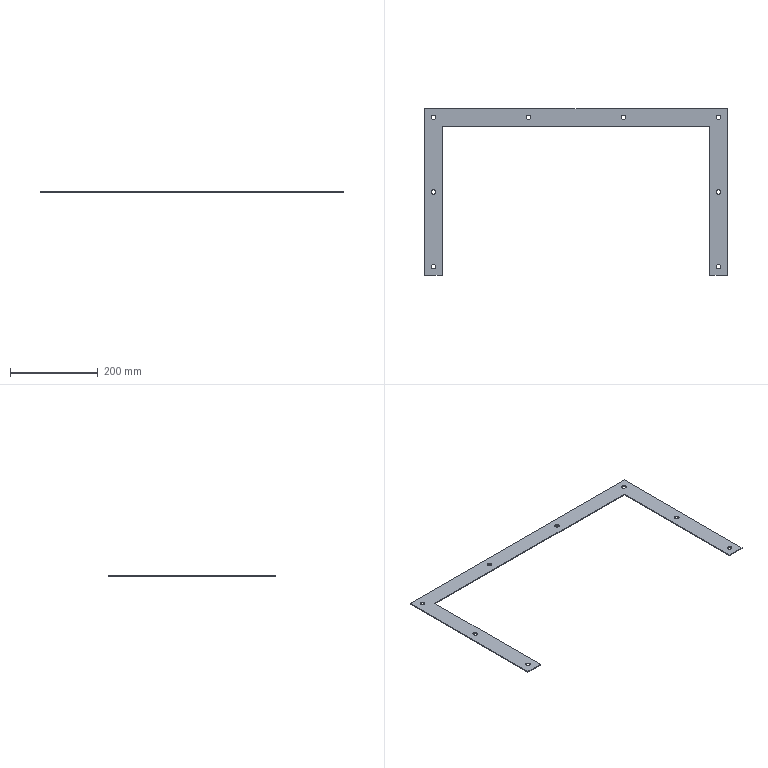Part | STEP file | 750038473 | 1 solid | 26 faces | box 690 x 380 x 2 mm | volume 108343 mm3 | cylinder 16 | plane 10 | commonest cylinder face diameters 10 x16
STEP:
#1=CARTESIAN_POINT('',(330.,275.,2.));
#2=VERTEX_POINT('',#1);
#3=CARTESIAN_POINT('',(320.,275.,2.));
#4=VERTEX_POINT('',#3);
#5=CARTESIAN_POINT('',(325.,275.,2.));
#6=DIRECTION('',(0.,0.,-1.));
#7=DIRECTION('',(-1.,0.,0.));
#8=AXIS2_PLACEMENT_3D('',#5,#6,#7);
#9=CIRCLE('',#8,5.);
#10=EDGE_CURVE('',#2,#4,#9,.T.);
#11=ORIENTED_EDGE('',*,*,#10,.F.);
#12=CARTESIAN_POINT('',(330.,275.,0.));
#13=VERTEX_POINT('',#12);
#14=CARTESIAN_POINT('',(330.,275.,787.721));
#15=DIRECTION('',(0.,0.,-1.));
#16=VECTOR('',#15,1000.);
#17=LINE('',#14,#16);
#18=EDGE_CURVE('',#2,#13,#17,.T.);
#19=ORIENTED_EDGE('',*,*,#18,.T.);
#20=CARTESIAN_POINT('',(320.,275.,0.));
#21=VERTEX_POINT('',#20);
#22=CARTESIAN_POINT('',(325.,275.,0.));
#23=DIRECTION('',(0.,0.,1.));
#24=DIRECTION('',(-1.,0.,0.));
#25=AXIS2_PLACEMENT_3D('',#22,#23,#24);
#26=CIRCLE('',#25,5.);
#27=EDGE_CURVE('',#21,#13,#26,.T.);
#28=ORIENTED_EDGE('',*,*,#27,.F.);
#29=CARTESIAN_POINT('',(320.,275.,787.721));
#30=DIRECTION('',(0.,0.,-1.));
#31=VECTOR('',#30,1000.);
#32=LINE('',#29,#31);
#33=EDGE_CURVE('',#4,#21,#32,.T.);
#34=ORIENTED_EDGE('',*,*,#33,.F.);
#35=EDGE_LOOP('',(#11,#19,#28,#34));
#36=FACE_OUTER_BOUND('',#35,.T.);
#37=CARTESIAN_POINT('',(325.,275.,787.721));
#38=DIRECTION('',(0.,0.,-1.));
#39=DIRECTION('',(-1.,0.,0.));
#40=AXIS2_PLACEMENT_3D('',#37,#38,#39);
#41=CYLINDRICAL_SURFACE('',#40,5.);
#42=ADVANCED_FACE('',(#36),#41,.F.);
#43=CARTESIAN_POINT('',(330.,105.,2.));
#44=VERTEX_POINT('',#43);
#45=CARTESIAN_POINT('',(320.,105.,2.));
#46=VERTEX_POINT('',#45);
#47=CARTESIAN_POINT('',(325.,105.,2.));
#48=DIRECTION('',(0.,0.,-1.));
#49=DIRECTION('',(-1.,0.,0.));
#50=AXIS2_PLACEMENT_3D('',#47,#48,#49);
#51=CIRCLE('',#50,5.);
#52=EDGE_CURVE('',#44,#46,#51,.T.);
#53=ORIENTED_EDGE('',*,*,#52,.F.);
#54=CARTESIAN_POINT('',(330.,105.,0.));
#55=VERTEX_POINT('',#54);
#56=CARTESIAN_POINT('',(330.,105.,787.721));
#57=DIRECTION('',(0.,0.,-1.));
#58=VECTOR('',#57,1000.);
#59=LINE('',#56,#58);
#60=EDGE_CURVE('',#44,#55,#59,.T.);
#61=ORIENTED_EDGE('',*,*,#60,.T.);
#62=CARTESIAN_POINT('',(320.,105.,0.));
#63=VERTEX_POINT('',#62);
#64=CARTESIAN_POINT('',(325.,105.,0.));
#65=DIRECTION('',(0.,0.,1.));
#66=DIRECTION('',(-1.,0.,0.));
#67=AXIS2_PLACEMENT_3D('',#64,#65,#66);
#68=CIRCLE('',#67,5.);
#69=EDGE_CURVE('',#63,#55,#68,.T.);
#70=ORIENTED_EDGE('',*,*,#69,.F.);
#71=CARTESIAN_POINT('',(320.,105.,787.721));
#72=DIRECTION('',(0.,0.,-1.));
#73=VECTOR('',#72,1000.);
#74=LINE('',#71,#73);
#75=EDGE_CURVE('',#46,#63,#74,.T.);
#76=ORIENTED_EDGE('',*,*,#75,.F.);
#77=EDGE_LOOP('',(#53,#61,#70,#76));
#78=FACE_OUTER_BOUND('',#77,.T.);
#79=CARTESIAN_POINT('',(325.,105.,787.721));
#80=DIRECTION('',(0.,0.,-1.));
#81=DIRECTION('',(-1.,0.,0.));
#82=AXIS2_PLACEMENT_3D('',#79,#80,#81);
#83=CYLINDRICAL_SURFACE('',#82,5.);
#84=ADVANCED_FACE('',(#78),#83,.F.);
#85=CARTESIAN_POINT('',(330.,-65.,2.));
#86=VERTEX_POINT('',#85);
#87=CARTESIAN_POINT('',(320.,-65.,2.));
#88=VERTEX_POINT('',#87);
#89=CARTESIAN_POINT('',(325.,-65.,2.));
#90=DIRECTION('',(0.,0.,-1.));
#91=DIRECTION('',(-1.,0.,0.));
#92=AXIS2_PLACEMENT_3D('',#89,#90,#91);
#93=CIRCLE('',#92,5.);
#94=EDGE_CURVE('',#86,#88,#93,.T.);
#95=ORIENTED_EDGE('',*,*,#94,.F.);
#96=CARTESIAN_POINT('',(330.,-65.,0.));
#97=VERTEX_POINT('',#96);
#98=CARTESIAN_POINT('',(330.,-65.,787.721));
#99=DIRECTION('',(0.,0.,-1.));
#100=VECTOR('',#99,1000.);
#101=LINE('',#98,#100);
#102=EDGE_CURVE('',#86,#97,#101,.T.);
#103=ORIENTED_EDGE('',*,*,#102,.T.);
#104=CARTESIAN_POINT('',(320.,-65.,0.));
#105=VERTEX_POINT('',#104);
#106=CARTESIAN_POINT('',(325.,-65.,0.));
#107=DIRECTION('',(0.,0.,1.));
#108=DIRECTION('',(-1.,0.,0.));
#109=AXIS2_PLACEMENT_3D('',#106,#107,#108);
#110=CIRCLE('',#109,5.);
#111=EDGE_CURVE('',#105,#97,#110,.T.);
#112=ORIENTED_EDGE('',*,*,#111,.F.);
#113=CARTESIAN_POINT('',(320.,-65.,787.721));
#114=DIRECTION('',(0.,0.,-1.));
#115=VECTOR('',#114,1000.);
#116=LINE('',#113,#115);
#117=EDGE_CURVE('',#88,#105,#116,.T.);
#118=ORIENTED_EDGE('',*,*,#117,.F.);
#119=EDGE_LOOP('',(#95,#103,#112,#118));
#120=FACE_OUTER_BOUND('',#119,.T.);
#121=CARTESIAN_POINT('',(325.,-65.,787.721));
#122=DIRECTION('',(0.,0.,-1.));
#123=DIRECTION('',(-1.,0.,0.));
#124=AXIS2_PLACEMENT_3D('',#121,#122,#123);
#125=CYLINDRICAL_SURFACE('',#124,5.);
#126=ADVANCED_FACE('',(#120),#125,.F.);
#127=CARTESIAN_POINT('',(113.333,275.,2.));
#128=VERTEX_POINT('',#127);
#129=CARTESIAN_POINT('',(103.333,275.,2.));
#130=VERTEX_POINT('',#129);
#131=CARTESIAN_POINT('',(108.333,275.,2.));
#132=DIRECTION('',(0.,0.,-1.));
#133=DIRECTION('',(-1.,0.,0.));
#134=AXIS2_PLACEMENT_3D('',#131,#132,#133);
#135=CIRCLE('',#134,5.);
#136=EDGE_CURVE('',#128,#130,#135,.T.);
#137=ORIENTED_EDGE('',*,*,#136,.F.);
#138=CARTESIAN_POINT('',(113.333,275.,0.));
#139=VERTEX_POINT('',#138);
#140=CARTESIAN_POINT('',(113.333,275.,787.721));
#141=DIRECTION('',(0.,0.,-1.));
#142=VECTOR('',#141,1000.);
#143=LINE('',#140,#142);
#144=EDGE_CURVE('',#128,#139,#143,.T.);
#145=ORIENTED_EDGE('',*,*,#144,.T.);
#146=CARTESIAN_POINT('',(103.333,275.,0.));
#147=VERTEX_POINT('',#146);
#148=CARTESIAN_POINT('',(108.333,275.,0.));
#149=DIRECTION('',(0.,0.,1.));
#150=DIRECTION('',(-1.,0.,0.));
#151=AXIS2_PLACEMENT_3D('',#148,#149,#150);
#152=CIRCLE('',#151,5.);
#153=EDGE_CURVE('',#147,#139,#152,.T.);
#154=ORIENTED_EDGE('',*,*,#153,.F.);
#155=CARTESIAN_POINT('',(103.333,275.,787.721));
#156=DIRECTION('',(0.,0.,-1.));
#157=VECTOR('',#156,1000.);
#158=LINE('',#155,#157);
#159=EDGE_CURVE('',#130,#147,#158,.T.);
#160=ORIENTED_EDGE('',*,*,#159,.F.);
#161=EDGE_LOOP('',(#137,#145,#154,#160));
#162=FACE_OUTER_BOUND('',#161,.T.);
#163=CARTESIAN_POINT('',(108.333,275.,787.721));
#164=DIRECTION('',(0.,0.,-1.));
#165=DIRECTION('',(-1.,0.,0.));
#166=AXIS2_PLACEMENT_3D('',#163,#164,#165);
#167=CYLINDRICAL_SURFACE('',#166,5.);
#168=ADVANCED_FACE('',(#162),#167,.F.);
#169=CARTESIAN_POINT('',(-103.333,275.,2.));
#170=VERTEX_POINT('',#169);
#171=CARTESIAN_POINT('',(-113.333,275.,2.));
#172=VERTEX_POINT('',#171);
#173=CARTESIAN_POINT('',(-108.333,275.,2.));
#174=DIRECTION('',(0.,0.,-1.));
#175=DIRECTION('',(-1.,0.,0.));
#176=AXIS2_PLACEMENT_3D('',#173,#174,#175);
#177=CIRCLE('',#176,5.);
#178=EDGE_CURVE('',#170,#172,#177,.T.);
#179=ORIENTED_EDGE('',*,*,#178,.F.);
#180=CARTESIAN_POINT('',(-103.333,275.,0.));
#181=VERTEX_POINT('',#180);
#182=CARTESIAN_POINT('',(-103.333,275.,787.721));
#183=DIRECTION('',(0.,0.,-1.));
#184=VECTOR('',#183,1000.);
#185=LINE('',#182,#184);
#186=EDGE_CURVE('',#170,#181,#185,.T.);
#187=ORIENTED_EDGE('',*,*,#186,.T.);
#188=CARTESIAN_POINT('',(-113.333,275.,0.));
#189=VERTEX_POINT('',#188);
#190=CARTESIAN_POINT('',(-108.333,275.,0.));
#191=DIRECTION('',(0.,0.,1.));
#192=DIRECTION('',(-1.,0.,0.));
#193=AXIS2_PLACEMENT_3D('',#190,#191,#192);
#194=CIRCLE('',#193,5.);
#195=EDGE_CURVE('',#189,#181,#194,.T.);
#196=ORIENTED_EDGE('',*,*,#195,.F.);
#197=CARTESIAN_POINT('',(-113.333,275.,787.721));
#198=DIRECTION('',(0.,0.,-1.));
#199=VECTOR('',#198,1000.);
#200=LINE('',#197,#199);
#201=EDGE_CURVE('',#172,#189,#200,.T.);
#202=ORIENTED_EDGE('',*,*,#201,.F.);
#203=EDGE_LOOP('',(#179,#187,#196,#202));
#204=FACE_OUTER_BOUND('',#203,.T.);
#205=CARTESIAN_POINT('',(-108.333,275.,787.721));
#206=DIRECTION('',(0.,0.,-1.));
#207=DIRECTION('',(-1.,0.,0.));
#208=AXIS2_PLACEMENT_3D('',#205,#206,#207);
#209=CYLINDRICAL_SURFACE('',#208,5.);
#210=ADVANCED_FACE('',(#204),#209,.F.);
#211=CARTESIAN_POINT('',(-320.,275.,2.));
#212=VERTEX_POINT('',#211);
#213=CARTESIAN_POINT('',(-330.,275.,2.));
#214=VERTEX_POINT('',#213);
#215=CARTESIAN_POINT('',(-325.,275.,2.));
#216=DIRECTION('',(0.,0.,-1.));
#217=DIRECTION('',(-1.,0.,0.));
#218=AXIS2_PLACEMENT_3D('',#215,#216,#217);
#219=CIRCLE('',#218,5.);
#220=EDGE_CURVE('',#212,#214,#219,.T.);
#221=ORIENTED_EDGE('',*,*,#220,.F.);
#222=CARTESIAN_POINT('',(-320.,275.,0.));
#223=VERTEX_POINT('',#222);
#224=CARTESIAN_POINT('',(-320.,275.,787.721));
#225=DIRECTION('',(0.,0.,-1.));
#226=VECTOR('',#225,1000.);
#227=LINE('',#224,#226);
#228=EDGE_CURVE('',#212,#223,#227,.T.);
#229=ORIENTED_EDGE('',*,*,#228,.T.);
#230=CARTESIAN_POINT('',(-330.,275.,0.));
#231=VERTEX_POINT('',#230);
#232=CARTESIAN_POINT('',(-325.,275.,0.));
#233=DIRECTION('',(0.,0.,1.));
#234=DIRECTION('',(-1.,0.,0.));
#235=AXIS2_PLACEMENT_3D('',#232,#233,#234);
#236=CIRCLE('',#235,5.);
#237=EDGE_CURVE('',#231,#223,#236,.T.);
#238=ORIENTED_EDGE('',*,*,#237,.F.);
#239=CARTESIAN_POINT('',(-330.,275.,787.721));
#240=DIRECTION('',(0.,0.,-1.));
#241=VECTOR('',#240,1000.);
#242=LINE('',#239,#241);
#243=EDGE_CURVE('',#214,#231,#242,.T.);
#244=ORIENTED_EDGE('',*,*,#243,.F.);
#245=EDGE_LOOP('',(#221,#229,#238,#244));
#246=FACE_OUTER_BOUND('',#245,.T.);
#247=CARTESIAN_POINT('',(-325.,275.,787.721));
#248=DIRECTION('',(0.,0.,-1.));
#249=DIRECTION('',(-1.,0.,0.));
#250=AXIS2_PLACEMENT_3D('',#247,#248,#249);
#251=CYLINDRICAL_SURFACE('',#250,5.);
#252=ADVANCED_FACE('',(#246),#251,.F.);
#253=CARTESIAN_POINT('',(-320.,105.,2.));
#254=VERTEX_POINT('',#253);
#255=CARTESIAN_POINT('',(-330.,105.,2.));
#256=VERTEX_POINT('',#255);
#257=CARTESIAN_POINT('',(-325.,105.,2.));
#258=DIRECTION('',(0.,0.,-1.));
#259=DIRECTION('',(-1.,0.,0.));
#260=AXIS2_PLACEMENT_3D('',#257,#258,#259);
#261=CIRCLE('',#260,5.);
#262=EDGE_CURVE('',#254,#256,#261,.T.);
#263=ORIENTED_EDGE('',*,*,#262,.F.);
#264=CARTESIAN_POINT('',(-320.,105.,0.));
#265=VERTEX_POINT('',#264);
#266=CARTESIAN_POINT('',(-320.,105.,787.721));
#267=DIRECTION('',(0.,0.,-1.));
#268=VECTOR('',#267,1000.);
#269=LINE('',#266,#268);
#270=EDGE_CURVE('',#254,#265,#269,.T.);
#271=ORIENTED_EDGE('',*,*,#270,.T.);
#272=CARTESIAN_POINT('',(-330.,105.,0.));
#273=VERTEX_POINT('',#272);
#274=CARTESIAN_POINT('',(-325.,105.,0.));
#275=DIRECTION('',(0.,0.,1.));
#276=DIRECTION('',(-1.,0.,0.));
#277=AXIS2_PLACEMENT_3D('',#274,#275,#276);
#278=CIRCLE('',#277,5.);
#279=EDGE_CURVE('',#273,#265,#278,.T.);
#280=ORIENTED_EDGE('',*,*,#279,.F.);
#281=CARTESIAN_POINT('',(-330.,105.,787.721));
#282=DIRECTION('',(0.,0.,-1.));
#283=VECTOR('',#282,1000.);
#284=LINE('',#281,#283);
#285=EDGE_CURVE('',#256,#273,#284,.T.);
#286=ORIENTED_EDGE('',*,*,#285,.F.);
#287=EDGE_LOOP('',(#263,#271,#280,#286));
#288=FACE_OUTER_BOUND('',#287,.T.);
#289=CARTESIAN_POINT('',(-325.,105.,787.721));
#290=DIRECTION('',(0.,0.,-1.));
#291=DIRECTION('',(-1.,0.,0.));
#292=AXIS2_PLACEMENT_3D('',#289,#290,#291);
#293=CYLINDRICAL_SURFACE('',#292,5.);
#294=ADVANCED_FACE('',(#288),#293,.F.);
#295=CARTESIAN_POINT('',(-320.,-65.,2.));
#296=VERTEX_POINT('',#295);
#297=CARTESIAN_POINT('',(-330.,-65.,2.));
#298=VERTEX_POINT('',#297);
#299=CARTESIAN_POINT('',(-325.,-65.,2.));
#300=DIRECTION('',(0.,0.,-1.));
#301=DIRECTION('',(-1.,0.,0.));
#302=AXIS2_PLACEMENT_3D('',#299,#300,#301);
#303=CIRCLE('',#302,5.);
#304=EDGE_CURVE('',#296,#298,#303,.T.);
#305=ORIENTED_EDGE('',*,*,#304,.F.);
#306=CARTESIAN_POINT('',(-320.,-65.,0.));
#307=VERTEX_POINT('',#306);
#308=CARTESIAN_POINT('',(-320.,-65.,787.721));
#309=DIRECTION('',(0.,0.,-1.));
#310=VECTOR('',#309,1000.);
#311=LINE('',#308,#310);
#312=EDGE_CURVE('',#296,#307,#311,.T.);
#313=ORIENTED_EDGE('',*,*,#312,.T.);
#314=CARTESIAN_POINT('',(-330.,-65.,0.));
#315=VERTEX_POINT('',#314);
#316=CARTESIAN_POINT('',(-325.,-65.,0.));
#317=DIRECTION('',(0.,0.,1.));
#318=DIRECTION('',(-1.,0.,0.));
#319=AXIS2_PLACEMENT_3D('',#316,#317,#318);
#320=CIRCLE('',#319,5.);
#321=EDGE_CURVE('',#315,#307,#320,.T.);
#322=ORIENTED_EDGE('',*,*,#321,.F.);
#323=CARTESIAN_POINT('',(-330.,-65.,787.721));
#324=DIRECTION('',(0.,0.,-1.));
#325=VECTOR('',#324,1000.);
#326=LINE('',#323,#325);
#327=EDGE_CURVE('',#298,#315,#326,.T.);
#328=ORIENTED_EDGE('',*,*,#327,.F.);
#329=EDGE_LOOP('',(#305,#313,#322,#328));
#330=FACE_OUTER_BOUND('',#329,.T.);
#331=CARTESIAN_POINT('',(-325.,-65.,787.721));
#332=DIRECTION('',(0.,0.,-1.));
#333=DIRECTION('',(-1.,0.,0.));
#334=AXIS2_PLACEMENT_3D('',#331,#332,#333);
#335=CYLINDRICAL_SURFACE('',#334,5.);
#336=ADVANCED_FACE('',(#330),#335,.F.);
#337=CARTESIAN_POINT('',(305.,-85.,2.));
#338=VERTEX_POINT('',#337);
#339=CARTESIAN_POINT('',(345.,-85.,2.));
#340=VERTEX_POINT('',#339);
#341=CARTESIAN_POINT('',(0.,-85.,2.));
#342=DIRECTION('',(1.,0.,0.));
#343=VECTOR('',#342,1000.);
#344=LINE('',#341,#343);
#345=EDGE_CURVE('',#338,#340,#344,.T.);
#346=ORIENTED_EDGE('',*,*,#345,.T.);
#347=CARTESIAN_POINT('',(345.,295.,2.));
#348=VERTEX_POINT('',#347);
#349=CARTESIAN_POINT('',(345.,0.,2.));
#350=DIRECTION('',(0.,1.,0.));
#351=VECTOR('',#350,1000.);
#352=LINE('',#349,#351);
#353=EDGE_CURVE('',#340,#348,#352,.T.);
#354=ORIENTED_EDGE('',*,*,#353,.T.);
#355=CARTESIAN_POINT('',(-345.,295.,2.));
#356=VERTEX_POINT('',#355);
#357=CARTESIAN_POINT('',(0.,295.,2.));
#358=DIRECTION('',(-1.,0.,0.));
#359=VECTOR('',#358,1000.);
#360=LINE('',#357,#359);
#361=EDGE_CURVE('',#348,#356,#360,.T.);
#362=ORIENTED_EDGE('',*,*,#361,.T.);
#363=CARTESIAN_POINT('',(-345.,-85.,2.));
#364=VERTEX_POINT('',#363);
#365=CARTESIAN_POINT('',(-345.,0.,2.));
#366=DIRECTION('',(0.,-1.,0.));
#367=VECTOR('',#366,1000.);
#368=LINE('',#365,#367);
#369=EDGE_CURVE('',#356,#364,#368,.T.);
#370=ORIENTED_EDGE('',*,*,#369,.T.);
#371=CARTESIAN_POINT('',(-305.,-85.,2.));
#372=VERTEX_POINT('',#371);
#373=CARTESIAN_POINT('',(0.,-85.,2.));
#374=DIRECTION('',(1.,0.,0.));
#375=VECTOR('',#374,1000.);
#376=LINE('',#373,#375);
#377=EDGE_CURVE('',#364,#372,#376,.T.);
#378=ORIENTED_EDGE('',*,*,#377,.T.);
#379=CARTESIAN_POINT('',(-305.,255.,2.));
#380=VERTEX_POINT('',#379);
#381=CARTESIAN_POINT('',(-305.,0.,2.));
#382=DIRECTION('',(0.,1.,0.));
#383=VECTOR('',#382,1000.);
#384=LINE('',#381,#383);
#385=EDGE_CURVE('',#372,#380,#384,.T.);
#386=ORIENTED_EDGE('',*,*,#385,.T.);
#387=CARTESIAN_POINT('',(305.,255.,2.));
#388=VERTEX_POINT('',#387);
#389=CARTESIAN_POINT('',(0.,255.,2.));
#390=DIRECTION('',(1.,0.,0.));
#391=VECTOR('',#390,1000.);
#392=LINE('',#389,#391);
#393=EDGE_CURVE('',#380,#388,#392,.T.);
#394=ORIENTED_EDGE('',*,*,#393,.T.);
#395=CARTESIAN_POINT('',(305.,0.,2.));
#396=DIRECTION('',(0.,-1.,0.));
#397=VECTOR('',#396,1000.);
#398=LINE('',#395,#397);
#399=EDGE_CURVE('',#388,#338,#398,.T.);
#400=ORIENTED_EDGE('',*,*,#399,.T.);
#401=EDGE_LOOP('',(#346,#354,#362,#370,#378,#386,#394,#400));
#402=FACE_OUTER_BOUND('',#401,.T.);
#403=CARTESIAN_POINT('',(325.,275.,2.));
#404=DIRECTION('',(0.,0.,-1.));
#405=DIRECTION('',(-1.,0.,0.));
#406=AXIS2_PLACEMENT_3D('',#403,#404,#405);
#407=CIRCLE('',#406,5.);
#408=EDGE_CURVE('',#4,#2,#407,.T.);
#409=ORIENTED_EDGE('',*,*,#408,.T.);
#410=ORIENTED_EDGE('',*,*,#10,.T.);
#411=EDGE_LOOP('',(#409,#410));
#412=FACE_BOUND('',#411,.T.);
#413=CARTESIAN_POINT('',(325.,105.,2.));
#414=DIRECTION('',(0.,0.,-1.));
#415=DIRECTION('',(-1.,0.,0.));
#416=AXIS2_PLACEMENT_3D('',#413,#414,#415);
#417=CIRCLE('',#416,5.);
#418=EDGE_CURVE('',#46,#44,#417,.T.);
#419=ORIENTED_EDGE('',*,*,#418,.T.);
#420=ORIENTED_EDGE('',*,*,#52,.T.);
#421=EDGE_LOOP('',(#419,#420));
#422=FACE_BOUND('',#421,.T.);
#423=CARTESIAN_POINT('',(325.,-65.,2.));
#424=DIRECTION('',(0.,0.,-1.));
#425=DIRECTION('',(-1.,0.,0.));
#426=AXIS2_PLACEMENT_3D('',#423,#424,#425);
#427=CIRCLE('',#426,5.);
#428=EDGE_CURVE('',#88,#86,#427,.T.);
#429=ORIENTED_EDGE('',*,*,#428,.T.);
#430=ORIENTED_EDGE('',*,*,#94,.T.);
#431=EDGE_LOOP('',(#429,#430));
#432=FACE_BOUND('',#431,.T.);
#433=CARTESIAN_POINT('',(108.333,275.,2.));
#434=DIRECTION('',(0.,0.,-1.));
#435=DIRECTION('',(-1.,0.,0.));
#436=AXIS2_PLACEMENT_3D('',#433,#434,#435);
#437=CIRCLE('',#436,5.);
#438=EDGE_CURVE('',#130,#128,#437,.T.);
#439=ORIENTED_EDGE('',*,*,#438,.T.);
#440=ORIENTED_EDGE('',*,*,#136,.T.);
#441=EDGE_LOOP('',(#439,#440));
#442=FACE_BOUND('',#441,.T.);
#443=CARTESIAN_POINT('',(-108.333,275.,2.));
#444=DIRECTION('',(0.,0.,-1.));
#445=DIRECTION('',(-1.,0.,0.));
#446=AXIS2_PLACEMENT_3D('',#443,#444,#445);
#447=CIRCLE('',#446,5.);
#448=EDGE_CURVE('',#172,#170,#447,.T.);
#449=ORIENTED_EDGE('',*,*,#448,.T.);
#450=ORIENTED_EDGE('',*,*,#178,.T.);
#451=EDGE_LOOP('',(#449,#450));
#452=FACE_BOUND('',#451,.T.);
#453=CARTESIAN_POINT('',(-325.,275.,2.));
#454=DIRECTION('',(0.,0.,-1.));
#455=DIRECTION('',(-1.,0.,0.));
#456=AXIS2_PLACEMENT_3D('',#453,#454,#455);
#457=CIRCLE('',#456,5.);
#458=EDGE_CURVE('',#214,#212,#457,.T.);
#459=ORIENTED_EDGE('',*,*,#458,.T.);
#460=ORIENTED_EDGE('',*,*,#220,.T.);
#461=EDGE_LOOP('',(#459,#460));
#462=FACE_BOUND('',#461,.T.);
#463=CARTESIAN_POINT('',(-325.,105.,2.));
#464=DIRECTION('',(0.,0.,-1.));
#465=DIRECTION('',(-1.,0.,0.));
#466=AXIS2_PLACEMENT_3D('',#463,#464,#465);
#467=CIRCLE('',#466,5.);
#468=EDGE_CURVE('',#256,#254,#467,.T.);
#469=ORIENTED_EDGE('',*,*,#468,.T.);
#470=ORIENTED_EDGE('',*,*,#262,.T.);
#471=EDGE_LOOP('',(#469,#470));
#472=FACE_BOUND('',#471,.T.);
#473=CARTESIAN_POINT('',(-325.,-65.,2.));
#474=DIRECTION('',(0.,0.,-1.));
#475=DIRECTION('',(-1.,0.,0.));
#476=AXIS2_PLACEMENT_3D('',#473,#474,#475);
#477=CIRCLE('',#476,5.);
#478=EDGE_CURVE('',#298,#296,#477,.T.);
#479=ORIENTED_EDGE('',*,*,#478,.T.);
#480=ORIENTED_EDGE('',*,*,#304,.T.);
#481=EDGE_LOOP('',(#479,#480));
#482=FACE_BOUND('',#481,.T.);
#483=CARTESIAN_POINT('',(0.,0.,2.));
#484=DIRECTION('',(0.,0.,1.));
#485=DIRECTION('',(1.,0.,0.));
#486=AXIS2_PLACEMENT_3D('',#483,#484,#485);
#487=PLANE('',#486);
#488=ADVANCED_FACE('',(#402,#412,#422,#432,#442,#452,#462,#472,#482),#487,.T.);
#489=CARTESIAN_POINT('',(345.,295.,0.));
#490=VERTEX_POINT('',#489);
#491=CARTESIAN_POINT('',(345.,295.,2.));
#492=DIRECTION('',(0.,0.,-1.));
#493=VECTOR('',#492,1000.);
#494=LINE('',#491,#493);
#495=EDGE_CURVE('',#348,#490,#494,.T.);
#496=ORIENTED_EDGE('',*,*,#495,.F.);
#497=ORIENTED_EDGE('',*,*,#353,.F.);
#498=CARTESIAN_POINT('',(345.,-85.,0.));
#499=VERTEX_POINT('',#498);
#500=CARTESIAN_POINT('',(345.,-85.,2.));
#501=DIRECTION('',(0.,0.,1.));
#502=VECTOR('',#501,1000.);
#503=LINE('',#500,#502);
#504=EDGE_CURVE('',#499,#340,#503,.T.);
#505=ORIENTED_EDGE('',*,*,#504,.F.);
#506=CARTESIAN_POINT('',(345.,-85.,0.));
#507=DIRECTION('',(0.,-1.,0.));
#508=VECTOR('',#507,1000.);
#509=LINE('',#506,#508);
#510=EDGE_CURVE('',#490,#499,#509,.T.);
#511=ORIENTED_EDGE('',*,*,#510,.F.);
#512=EDGE_LOOP('',(#496,#497,#505,#511));
#513=FACE_OUTER_BOUND('',#512,.T.);
#514=CARTESIAN_POINT('',(345.,-85.,2.));
#515=DIRECTION('',(-1.,0.,0.));
#516=DIRECTION('',(0.,-1.,0.));
#517=AXIS2_PLACEMENT_3D('',#514,#515,#516);
#518=PLANE('',#517);
#519=ADVANCED_FACE('',(#513),#518,.F.);
#520=ORIENTED_EDGE('',*,*,#504,.T.);
#521=ORIENTED_EDGE('',*,*,#345,.F.);
#522=CARTESIAN_POINT('',(305.,-85.,0.));
#523=VERTEX_POINT('',#522);
#524=CARTESIAN_POINT('',(305.,-85.,2.));
#525=DIRECTION('',(0.,0.,1.));
#526=VECTOR('',#525,1000.);
#527=LINE('',#524,#526);
#528=EDGE_CURVE('',#523,#338,#527,.T.);
#529=ORIENTED_EDGE('',*,*,#528,.F.);
#530=CARTESIAN_POINT('',(305.,-85.,0.));
#531=DIRECTION('',(-1.,0.,0.));
#532=VECTOR('',#531,1000.);
#533=LINE('',#530,#532);
#534=EDGE_CURVE('',#499,#523,#533,.T.);
#535=ORIENTED_EDGE('',*,*,#534,.F.);
#536=EDGE_LOOP('',(#520,#521,#529,#535));
#537=FACE_OUTER_BOUND('',#536,.T.);
#538=CARTESIAN_POINT('',(305.,-85.,2.));
#539=DIRECTION('',(0.,1.,0.));
#540=DIRECTION('',(0.,0.,1.));
#541=AXIS2_PLACEMENT_3D('',#538,#539,#540);
#542=PLANE('',#541);
#543=ADVANCED_FACE('',(#537),#542,.F.);
#544=ORIENTED_EDGE('',*,*,#528,.T.);
#545=ORIENTED_EDGE('',*,*,#399,.F.);
#546=CARTESIAN_POINT('',(305.,255.,0.));
#547=VERTEX_POINT('',#546);
#548=CARTESIAN_POINT('',(305.,255.,2.));
#549=DIRECTION('',(0.,0.,1.));
#550=VECTOR('',#549,1000.);
#551=LINE('',#548,#550);
#552=EDGE_CURVE('',#547,#388,#551,.T.);
#553=ORIENTED_EDGE('',*,*,#552,.F.);
#554=CARTESIAN_POINT('',(305.,255.,0.));
#555=DIRECTION('',(0.,1.,0.));
#556=VECTOR('',#555,1000.);
#557=LINE('',#554,#556);
#558=EDGE_CURVE('',#523,#547,#557,.T.);
#559=ORIENTED_EDGE('',*,*,#558,.F.);
#560=EDGE_LOOP('',(#544,#545,#553,#559));
#561=FACE_OUTER_BOUND('',#560,.T.);
#562=CARTESIAN_POINT('',(305.,255.,2.));
#563=DIRECTION('',(1.,0.,0.));
#564=DIRECTION('',(0.,1.,0.));
#565=AXIS2_PLACEMENT_3D('',#562,#563,#564);
#566=PLANE('',#565);
#567=ADVANCED_FACE('',(#561),#566,.F.);
#568=ORIENTED_EDGE('',*,*,#552,.T.);
#569=ORIENTED_EDGE('',*,*,#393,.F.);
#570=CARTESIAN_POINT('',(-305.,255.,0.));
#571=VERTEX_POINT('',#570);
#572=CARTESIAN_POINT('',(-305.,255.,2.));
#573=DIRECTION('',(0.,0.,1.));
#574=VECTOR('',#573,1000.);
#575=LINE('',#572,#574);
#576=EDGE_CURVE('',#571,#380,#575,.T.);
#577=ORIENTED_EDGE('',*,*,#576,.F.);
#578=CARTESIAN_POINT('',(-305.,255.,0.));
#579=DIRECTION('',(-1.,0.,0.));
#580=VECTOR('',#579,1000.);
#581=LINE('',#578,#580);
#582=EDGE_CURVE('',#547,#571,#581,.T.);
#583=ORIENTED_EDGE('',*,*,#582,.F.);
#584=EDGE_LOOP('',(#568,#569,#577,#583));
#585=FACE_OUTER_BOUND('',#584,.T.);
#586=CARTESIAN_POINT('',(-305.,255.,2.));
#587=DIRECTION('',(0.,1.,0.));
#588=DIRECTION('',(0.,0.,1.));
#589=AXIS2_PLACEMENT_3D('',#586,#587,#588);
#590=PLANE('',#589);
#591=ADVANCED_FACE('',(#585),#590,.F.);
#592=ORIENTED_EDGE('',*,*,#576,.T.);
#593=ORIENTED_EDGE('',*,*,#385,.F.);
#594=CARTESIAN_POINT('',(-305.,-85.,0.));
#595=VERTEX_POINT('',#594);
#596=CARTESIAN_POINT('',(-305.,-85.,2.));
#597=DIRECTION('',(0.,0.,1.));
#598=VECTOR('',#597,1000.);
#599=LINE('',#596,#598);
#600=EDGE_CURVE('',#595,#372,#599,.T.);
#601=ORIENTED_EDGE('',*,*,#600,.F.);
#602=CARTESIAN_POINT('',(-305.,-85.,0.));
#603=DIRECTION('',(0.,-1.,0.));
#604=VECTOR('',#603,1000.);
#605=LINE('',#602,#604);
#606=EDGE_CURVE('',#571,#595,#605,.T.);
#607=ORIENTED_EDGE('',*,*,#606,.F.);
#608=EDGE_LOOP('',(#592,#593,#601,#607));
#609=FACE_OUTER_BOUND('',#608,.T.);
#610=CARTESIAN_POINT('',(-305.,-85.,2.));
#611=DIRECTION('',(-1.,0.,0.));
#612=DIRECTION('',(0.,-1.,0.));
#613=AXIS2_PLACEMENT_3D('',#610,#611,#612);
#614=PLANE('',#613);
#615=ADVANCED_FACE('',(#609),#614,.F.);
#616=ORIENTED_EDGE('',*,*,#600,.T.);
#617=ORIENTED_EDGE('',*,*,#377,.F.);
#618=CARTESIAN_POINT('',(-345.,-85.,0.));
#619=VERTEX_POINT('',#618);
#620=CARTESIAN_POINT('',(-345.,-85.,2.));
#621=DIRECTION('',(0.,0.,1.));
#622=VECTOR('',#621,1000.);
#623=LINE('',#620,#622);
#624=EDGE_CURVE('',#619,#364,#623,.T.);
#625=ORIENTED_EDGE('',*,*,#624,.F.);
#626=CARTESIAN_POINT('',(-345.,-85.,0.));
#627=DIRECTION('',(-1.,0.,0.));
#628=VECTOR('',#627,1000.);
#629=LINE('',#626,#628);
#630=EDGE_CURVE('',#595,#619,#629,.T.);
#631=ORIENTED_EDGE('',*,*,#630,.F.);
#632=EDGE_LOOP('',(#616,#617,#625,#631));
#633=FACE_OUTER_BOUND('',#632,.T.);
#634=CARTESIAN_POINT('',(-345.,-85.,2.));
#635=DIRECTION('',(0.,1.,0.));
#636=DIRECTION('',(0.,0.,1.));
#637=AXIS2_PLACEMENT_3D('',#634,#635,#636);
#638=PLANE('',#637);
#639=ADVANCED_FACE('',(#633),#638,.F.);
#640=ORIENTED_EDGE('',*,*,#624,.T.);
#641=ORIENTED_EDGE('',*,*,#369,.F.);
#642=CARTESIAN_POINT('',(-345.,295.,0.));
#643=VERTEX_POINT('',#642);
#644=CARTESIAN_POINT('',(-345.,295.,2.));
#645=DIRECTION('',(0.,0.,1.));
#646=VECTOR('',#645,1000.);
#647=LINE('',#644,#646);
#648=EDGE_CURVE('',#643,#356,#647,.T.);
#649=ORIENTED_EDGE('',*,*,#648,.F.);
#650=CARTESIAN_POINT('',(-345.,295.,0.));
#651=DIRECTION('',(0.,1.,0.));
#652=VECTOR('',#651,1000.);
#653=LINE('',#650,#652);
#654=EDGE_CURVE('',#619,#643,#653,.T.);
#655=ORIENTED_EDGE('',*,*,#654,.F.);
#656=EDGE_LOOP('',(#640,#641,#649,#655));
#657=FACE_OUTER_BOUND('',#656,.T.);
#658=CARTESIAN_POINT('',(-345.,295.,2.));
#659=DIRECTION('',(1.,0.,0.));
#660=DIRECTION('',(0.,1.,0.));
#661=AXIS2_PLACEMENT_3D('',#658,#659,#660);
#662=PLANE('',#661);
#663=ADVANCED_FACE('',(#657),#662,.F.);
#664=ORIENTED_EDGE('',*,*,#648,.T.);
#665=ORIENTED_EDGE('',*,*,#361,.F.);
#666=ORIENTED_EDGE('',*,*,#495,.T.);
#667=CARTESIAN_POINT('',(345.,295.,0.));
#668=DIRECTION('',(1.,0.,0.));
#669=VECTOR('',#668,1000.);
#670=LINE('',#667,#669);
#671=EDGE_CURVE('',#643,#490,#670,.T.);
#672=ORIENTED_EDGE('',*,*,#671,.F.);
#673=EDGE_LOOP('',(#664,#665,#666,#672));
#674=FACE_OUTER_BOUND('',#673,.T.);
#675=CARTESIAN_POINT('',(345.,295.,2.));
#676=DIRECTION('',(0.,-1.,0.));
#677=DIRECTION('',(0.,0.,-1.));
#678=AXIS2_PLACEMENT_3D('',#675,#676,#677);
#679=PLANE('',#678);
#680=ADVANCED_FACE('',(#674),#679,.F.);
#681=ORIENTED_EDGE('',*,*,#18,.F.);
#682=ORIENTED_EDGE('',*,*,#408,.F.);
#683=ORIENTED_EDGE('',*,*,#33,.T.);
#684=CARTESIAN_POINT('',(325.,275.,0.));
#685=DIRECTION('',(0.,0.,1.));
#686=DIRECTION('',(-1.,0.,0.));
#687=AXIS2_PLACEMENT_3D('',#684,#685,#686);
#688=CIRCLE('',#687,5.);
#689=EDGE_CURVE('',#13,#21,#688,.T.);
#690=ORIENTED_EDGE('',*,*,#689,.F.);
#691=EDGE_LOOP('',(#681,#682,#683,#690));
#692=FACE_OUTER_BOUND('',#691,.T.);
#693=CARTESIAN_POINT('',(325.,275.,787.721));
#694=DIRECTION('',(0.,0.,-1.));
#695=DIRECTION('',(-1.,0.,0.));
#696=AXIS2_PLACEMENT_3D('',#693,#694,#695);
#697=CYLINDRICAL_SURFACE('',#696,5.);
#698=ADVANCED_FACE('',(#692),#697,.F.);
#699=ORIENTED_EDGE('',*,*,#60,.F.);
#700=ORIENTED_EDGE('',*,*,#418,.F.);
#701=ORIENTED_EDGE('',*,*,#75,.T.);
#702=CARTESIAN_POINT('',(325.,105.,0.));
#703=DIRECTION('',(0.,0.,1.));
#704=DIRECTION('',(-1.,0.,0.));
#705=AXIS2_PLACEMENT_3D('',#702,#703,#704);
#706=CIRCLE('',#705,5.);
#707=EDGE_CURVE('',#55,#63,#706,.T.);
#708=ORIENTED_EDGE('',*,*,#707,.F.);
#709=EDGE_LOOP('',(#699,#700,#701,#708));
#710=FACE_OUTER_BOUND('',#709,.T.);
#711=CARTESIAN_POINT('',(325.,105.,787.721));
#712=DIRECTION('',(0.,0.,-1.));
#713=DIRECTION('',(-1.,0.,0.));
#714=AXIS2_PLACEMENT_3D('',#711,#712,#713);
#715=CYLINDRICAL_SURFACE('',#714,5.);
#716=ADVANCED_FACE('',(#710),#715,.F.);
#717=ORIENTED_EDGE('',*,*,#102,.F.);
#718=ORIENTED_EDGE('',*,*,#428,.F.);
#719=ORIENTED_EDGE('',*,*,#117,.T.);
#720=CARTESIAN_POINT('',(325.,-65.,0.));
#721=DIRECTION('',(0.,0.,1.));
#722=DIRECTION('',(-1.,0.,0.));
#723=AXIS2_PLACEMENT_3D('',#720,#721,#722);
#724=CIRCLE('',#723,5.);
#725=EDGE_CURVE('',#97,#105,#724,.T.);
#726=ORIENTED_EDGE('',*,*,#725,.F.);
#727=EDGE_LOOP('',(#717,#718,#719,#726));
#728=FACE_OUTER_BOUND('',#727,.T.);
#729=CARTESIAN_POINT('',(325.,-65.,787.721));
#730=DIRECTION('',(0.,0.,-1.));
#731=DIRECTION('',(-1.,0.,0.));
#732=AXIS2_PLACEMENT_3D('',#729,#730,#731);
#733=CYLINDRICAL_SURFACE('',#732,5.);
#734=ADVANCED_FACE('',(#728),#733,.F.);
#735=ORIENTED_EDGE('',*,*,#144,.F.);
#736=ORIENTED_EDGE('',*,*,#438,.F.);
#737=ORIENTED_EDGE('',*,*,#159,.T.);
#738=CARTESIAN_POINT('',(108.333,275.,0.));
#739=DIRECTION('',(0.,0.,1.));
#740=DIRECTION('',(-1.,0.,0.));
#741=AXIS2_PLACEMENT_3D('',#738,#739,#740);
#742=CIRCLE('',#741,5.);
#743=EDGE_CURVE('',#139,#147,#742,.T.);
#744=ORIENTED_EDGE('',*,*,#743,.F.);
#745=EDGE_LOOP('',(#735,#736,#737,#744));
#746=FACE_OUTER_BOUND('',#745,.T.);
#747=CARTESIAN_POINT('',(108.333,275.,787.721));
#748=DIRECTION('',(0.,0.,-1.));
#749=DIRECTION('',(-1.,0.,0.));
#750=AXIS2_PLACEMENT_3D('',#747,#748,#749);
#751=CYLINDRICAL_SURFACE('',#750,5.);
#752=ADVANCED_FACE('',(#746),#751,.F.);
#753=ORIENTED_EDGE('',*,*,#186,.F.);
#754=ORIENTED_EDGE('',*,*,#448,.F.);
#755=ORIENTED_EDGE('',*,*,#201,.T.);
#756=CARTESIAN_POINT('',(-108.333,275.,0.));
#757=DIRECTION('',(0.,0.,1.));
#758=DIRECTION('',(-1.,0.,0.));
#759=AXIS2_PLACEMENT_3D('',#756,#757,#758);
#760=CIRCLE('',#759,5.);
#761=EDGE_CURVE('',#181,#189,#760,.T.);
#762=ORIENTED_EDGE('',*,*,#761,.F.);
#763=EDGE_LOOP('',(#753,#754,#755,#762));
#764=FACE_OUTER_BOUND('',#763,.T.);
#765=CARTESIAN_POINT('',(-108.333,275.,787.721));
#766=DIRECTION('',(0.,0.,-1.));
#767=DIRECTION('',(-1.,0.,0.));
#768=AXIS2_PLACEMENT_3D('',#765,#766,#767);
#769=CYLINDRICAL_SURFACE('',#768,5.);
#770=ADVANCED_FACE('',(#764),#769,.F.);
#771=ORIENTED_EDGE('',*,*,#228,.F.);
#772=ORIENTED_EDGE('',*,*,#458,.F.);
#773=ORIENTED_EDGE('',*,*,#243,.T.);
#774=CARTESIAN_POINT('',(-325.,275.,0.));
#775=DIRECTION('',(0.,0.,1.));
#776=DIRECTION('',(-1.,0.,0.));
#777=AXIS2_PLACEMENT_3D('',#774,#775,#776);
#778=CIRCLE('',#777,5.);
#779=EDGE_CURVE('',#223,#231,#778,.T.);
#780=ORIENTED_EDGE('',*,*,#779,.F.);
#781=EDGE_LOOP('',(#771,#772,#773,#780));
#782=FACE_OUTER_BOUND('',#781,.T.);
#783=CARTESIAN_POINT('',(-325.,275.,787.721));
#784=DIRECTION('',(0.,0.,-1.));
#785=DIRECTION('',(-1.,0.,0.));
#786=AXIS2_PLACEMENT_3D('',#783,#784,#785);
#787=CYLINDRICAL_SURFACE('',#786,5.);
#788=ADVANCED_FACE('',(#782),#787,.F.);
#789=ORIENTED_EDGE('',*,*,#270,.F.);
#790=ORIENTED_EDGE('',*,*,#468,.F.);
#791=ORIENTED_EDGE('',*,*,#285,.T.);
#792=CARTESIAN_POINT('',(-325.,105.,0.));
#793=DIRECTION('',(0.,0.,1.));
#794=DIRECTION('',(-1.,0.,0.));
#795=AXIS2_PLACEMENT_3D('',#792,#793,#794);
#796=CIRCLE('',#795,5.);
#797=EDGE_CURVE('',#265,#273,#796,.T.);
#798=ORIENTED_EDGE('',*,*,#797,.F.);
#799=EDGE_LOOP('',(#789,#790,#791,#798));
#800=FACE_OUTER_BOUND('',#799,.T.);
#801=CARTESIAN_POINT('',(-325.,105.,787.721));
#802=DIRECTION('',(0.,0.,-1.));
#803=DIRECTION('',(-1.,0.,0.));
#804=AXIS2_PLACEMENT_3D('',#801,#802,#803);
#805=CYLINDRICAL_SURFACE('',#804,5.);
#806=ADVANCED_FACE('',(#800),#805,.F.);
#807=ORIENTED_EDGE('',*,*,#312,.F.);
#808=ORIENTED_EDGE('',*,*,#478,.F.);
#809=ORIENTED_EDGE('',*,*,#327,.T.);
#810=CARTESIAN_POINT('',(-325.,-65.,0.));
#811=DIRECTION('',(0.,0.,1.));
#812=DIRECTION('',(-1.,0.,0.));
#813=AXIS2_PLACEMENT_3D('',#810,#811,#812);
#814=CIRCLE('',#813,5.);
#815=EDGE_CURVE('',#307,#315,#814,.T.);
#816=ORIENTED_EDGE('',*,*,#815,.F.);
#817=EDGE_LOOP('',(#807,#808,#809,#816));
#818=FACE_OUTER_BOUND('',#817,.T.);
#819=CARTESIAN_POINT('',(-325.,-65.,787.721));
#820=DIRECTION('',(0.,0.,-1.));
#821=DIRECTION('',(-1.,0.,0.));
#822=AXIS2_PLACEMENT_3D('',#819,#820,#821);
#823=CYLINDRICAL_SURFACE('',#822,5.);
#824=ADVANCED_FACE('',(#818),#823,.F.);
#825=ORIENTED_EDGE('',*,*,#510,.T.);
#826=ORIENTED_EDGE('',*,*,#534,.T.);
#827=ORIENTED_EDGE('',*,*,#558,.T.);
#828=ORIENTED_EDGE('',*,*,#582,.T.);
#829=ORIENTED_EDGE('',*,*,#606,.T.);
#830=ORIENTED_EDGE('',*,*,#630,.T.);
#831=ORIENTED_EDGE('',*,*,#654,.T.);
#832=ORIENTED_EDGE('',*,*,#671,.T.);
#833=EDGE_LOOP('',(#825,#826,#827,#828,#829,#830,#831,#832));
#834=FACE_OUTER_BOUND('',#833,.T.);
#835=ORIENTED_EDGE('',*,*,#27,.T.);
#836=ORIENTED_EDGE('',*,*,#689,.T.);
#837=EDGE_LOOP('',(#835,#836));
#838=FACE_BOUND('',#837,.T.);
#839=ORIENTED_EDGE('',*,*,#69,.T.);
#840=ORIENTED_EDGE('',*,*,#707,.T.);
#841=EDGE_LOOP('',(#839,#840));
#842=FACE_BOUND('',#841,.T.);
#843=ORIENTED_EDGE('',*,*,#111,.T.);
#844=ORIENTED_EDGE('',*,*,#725,.T.);
#845=EDGE_LOOP('',(#843,#844));
#846=FACE_BOUND('',#845,.T.);
#847=ORIENTED_EDGE('',*,*,#153,.T.);
#848=ORIENTED_EDGE('',*,*,#743,.T.);
#849=EDGE_LOOP('',(#847,#848));
#850=FACE_BOUND('',#849,.T.);
#851=ORIENTED_EDGE('',*,*,#195,.T.);
#852=ORIENTED_EDGE('',*,*,#761,.T.);
#853=EDGE_LOOP('',(#851,#852));
#854=FACE_BOUND('',#853,.T.);
#855=ORIENTED_EDGE('',*,*,#237,.T.);
#856=ORIENTED_EDGE('',*,*,#779,.T.);
#857=EDGE_LOOP('',(#855,#856));
#858=FACE_BOUND('',#857,.T.);
#859=ORIENTED_EDGE('',*,*,#279,.T.);
#860=ORIENTED_EDGE('',*,*,#797,.T.);
#861=EDGE_LOOP('',(#859,#860));
#862=FACE_BOUND('',#861,.T.);
#863=ORIENTED_EDGE('',*,*,#321,.T.);
#864=ORIENTED_EDGE('',*,*,#815,.T.);
#865=EDGE_LOOP('',(#863,#864));
#866=FACE_BOUND('',#865,.T.);
#867=CARTESIAN_POINT('',(0.,0.,0.));
#868=DIRECTION('',(0.,0.,1.));
#869=DIRECTION('',(1.,0.,0.));
#870=AXIS2_PLACEMENT_3D('',#867,#868,#869);
#871=PLANE('',#870);
#872=ADVANCED_FACE('',(#834,#838,#842,#846,#850,#854,#858,#862,#866),#871,.F.);
#873=CLOSED_SHELL('',(#42,#84,#126,#168,#210,#252,#294,#336,#488,#519,#543,#567,#591,#615,#639,#663,#680,#698,#716,#734,#752,#770,#788,#806,#824,#872));
#874=MANIFOLD_SOLID_BREP('',#873);
#875=CARTESIAN_POINT('',(0.,0.,0.));
#876=DIRECTION('',(0.,0.,1.));
#877=DIRECTION('',(1.,0.,0.));
#878=AXIS2_PLACEMENT_3D('',#875,#876,#877);
#879=(LENGTH_UNIT()NAMED_UNIT(*)SI_UNIT(.MILLI.,.METRE.));
#880=UNCERTAINTY_MEASURE_WITH_UNIT(LENGTH_MEASURE(0.00001),#879,'','');
#881=(NAMED_UNIT(*)PLANE_ANGLE_UNIT()SI_UNIT($,.RADIAN.));
#882=(NAMED_UNIT(*)SI_UNIT($,.STERADIAN.)SOLID_ANGLE_UNIT());
#883=(GEOMETRIC_REPRESENTATION_CONTEXT(3)GLOBAL_UNCERTAINTY_ASSIGNED_CONTEXT((#880))GLOBAL_UNIT_ASSIGNED_CONTEXT((#879,#881,#882))REPRESENTATION_CONTEXT('',''));
#884=ADVANCED_BREP_SHAPE_REPRESENTATION('',(#874,#878),#883);